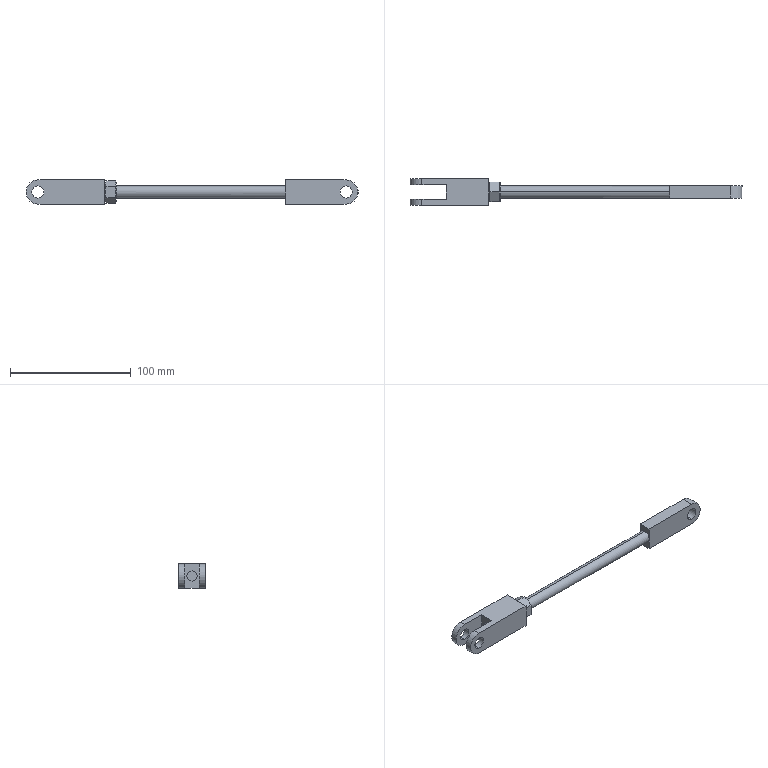Part | SolidWorks | features MirrorStock 1 | 3 solids | 42 faces | box 275 x 22 x 20 mm | volume 44683 mm3 | plane 23 | cylinder 15 | cone 4 | commonest cylinder face diameters 10 x8 20 x3 8.376 x2 8.5 x2
STEP:
#1=CARTESIAN_POINT('',(20.,0.,4.25));
#2=VERTEX_POINT('',#1);
#3=CARTESIAN_POINT('',(20.,0.,-4.25));
#4=VERTEX_POINT('',#3);
#5=CARTESIAN_POINT('',(20.,0.,0.));
#6=DIRECTION('',(-1.,0.,0.));
#7=DIRECTION('',(0.,0.,1.));
#8=AXIS2_PLACEMENT_3D('',#5,#6,#7);
#9=CIRCLE('',#8,4.25);
#10=EDGE_CURVE('',#2,#4,#9,.T.);
#11=ORIENTED_EDGE('',*,*,#10,.T.);
#12=CARTESIAN_POINT('',(55.,0.,-4.25));
#13=VERTEX_POINT('',#12);
#14=CARTESIAN_POINT('',(55.,0.,-4.25));
#15=DIRECTION('',(1.,0.,0.));
#16=VECTOR('',#15,1000.);
#17=LINE('',#14,#16);
#18=EDGE_CURVE('',#4,#13,#17,.T.);
#19=ORIENTED_EDGE('',*,*,#18,.T.);
#20=CARTESIAN_POINT('',(55.,0.,4.25));
#21=VERTEX_POINT('',#20);
#22=CARTESIAN_POINT('',(55.,0.,0.));
#23=DIRECTION('',(-1.,0.,0.));
#24=DIRECTION('',(0.,0.,1.));
#25=AXIS2_PLACEMENT_3D('',#22,#23,#24);
#26=CIRCLE('',#25,4.25);
#27=EDGE_CURVE('',#21,#13,#26,.T.);
#28=ORIENTED_EDGE('',*,*,#27,.F.);
#29=CARTESIAN_POINT('',(55.,0.,4.25));
#30=DIRECTION('',(1.,0.,0.));
#31=VECTOR('',#30,1000.);
#32=LINE('',#29,#31);
#33=EDGE_CURVE('',#2,#21,#32,.T.);
#34=ORIENTED_EDGE('',*,*,#33,.F.);
#35=EDGE_LOOP('',(#11,#19,#28,#34));
#36=FACE_OUTER_BOUND('',#35,.T.);
#37=CARTESIAN_POINT('',(55.,0.,0.));
#38=DIRECTION('',(1.,0.,0.));
#39=DIRECTION('',(0.,0.,1.));
#40=AXIS2_PLACEMENT_3D('',#37,#38,#39);
#41=CYLINDRICAL_SURFACE('',#40,4.25);
#42=ADVANCED_FACE('',(#36),#41,.F.);
#43=CARTESIAN_POINT('',(0.,11.,-5.));
#44=VERTEX_POINT('',#43);
#45=CARTESIAN_POINT('',(0.,11.,5.));
#46=VERTEX_POINT('',#45);
#47=CARTESIAN_POINT('',(0.,11.,0.));
#48=DIRECTION('',(0.,-1.,0.));
#49=DIRECTION('',(0.,0.,-1.));
#50=AXIS2_PLACEMENT_3D('',#47,#48,#49);
#51=CIRCLE('',#50,5.);
#52=EDGE_CURVE('',#44,#46,#51,.T.);
#53=ORIENTED_EDGE('',*,*,#52,.F.);
#54=CARTESIAN_POINT('',(0.,6.,-5.));
#55=VERTEX_POINT('',#54);
#56=CARTESIAN_POINT('',(0.,11.,-5.));
#57=DIRECTION('',(0.,-1.,0.));
#58=VECTOR('',#57,1000.);
#59=LINE('',#56,#58);
#60=EDGE_CURVE('',#44,#55,#59,.T.);
#61=ORIENTED_EDGE('',*,*,#60,.T.);
#62=CARTESIAN_POINT('',(0.,6.,5.));
#63=VERTEX_POINT('',#62);
#64=CARTESIAN_POINT('',(0.,6.,0.));
#65=DIRECTION('',(0.,-1.,0.));
#66=DIRECTION('',(0.,0.,-1.));
#67=AXIS2_PLACEMENT_3D('',#64,#65,#66);
#68=CIRCLE('',#67,5.);
#69=EDGE_CURVE('',#55,#63,#68,.T.);
#70=ORIENTED_EDGE('',*,*,#69,.T.);
#71=CARTESIAN_POINT('',(0.,11.,5.));
#72=DIRECTION('',(0.,-1.,0.));
#73=VECTOR('',#72,1000.);
#74=LINE('',#71,#73);
#75=EDGE_CURVE('',#46,#63,#74,.T.);
#76=ORIENTED_EDGE('',*,*,#75,.F.);
#77=EDGE_LOOP('',(#53,#61,#70,#76));
#78=FACE_OUTER_BOUND('',#77,.T.);
#79=CARTESIAN_POINT('',(0.,11.,0.));
#80=DIRECTION('',(0.,-1.,0.));
#81=DIRECTION('',(0.,0.,1.));
#82=AXIS2_PLACEMENT_3D('',#79,#80,#81);
#83=CYLINDRICAL_SURFACE('',#82,5.);
#84=ADVANCED_FACE('',(#78),#83,.F.);
#85=CARTESIAN_POINT('',(0.,-6.,5.));
#86=VERTEX_POINT('',#85);
#87=CARTESIAN_POINT('',(0.,-6.,-5.));
#88=VERTEX_POINT('',#87);
#89=CARTESIAN_POINT('',(0.,-6.,0.));
#90=DIRECTION('',(0.,1.,0.));
#91=DIRECTION('',(0.,0.,1.));
#92=AXIS2_PLACEMENT_3D('',#89,#90,#91);
#93=CIRCLE('',#92,5.);
#94=EDGE_CURVE('',#86,#88,#93,.T.);
#95=ORIENTED_EDGE('',*,*,#94,.T.);
#96=CARTESIAN_POINT('',(0.,-11.,-5.));
#97=VERTEX_POINT('',#96);
#98=CARTESIAN_POINT('',(0.,11.,-5.));
#99=DIRECTION('',(0.,-1.,0.));
#100=VECTOR('',#99,1000.);
#101=LINE('',#98,#100);
#102=EDGE_CURVE('',#88,#97,#101,.T.);
#103=ORIENTED_EDGE('',*,*,#102,.T.);
#104=CARTESIAN_POINT('',(0.,-11.,5.));
#105=VERTEX_POINT('',#104);
#106=CARTESIAN_POINT('',(0.,-11.,0.));
#107=DIRECTION('',(0.,-1.,0.));
#108=DIRECTION('',(0.,0.,-1.));
#109=AXIS2_PLACEMENT_3D('',#106,#107,#108);
#110=CIRCLE('',#109,5.);
#111=EDGE_CURVE('',#97,#105,#110,.T.);
#112=ORIENTED_EDGE('',*,*,#111,.T.);
#113=CARTESIAN_POINT('',(0.,11.,5.));
#114=DIRECTION('',(0.,-1.,0.));
#115=VECTOR('',#114,1000.);
#116=LINE('',#113,#115);
#117=EDGE_CURVE('',#86,#105,#116,.T.);
#118=ORIENTED_EDGE('',*,*,#117,.F.);
#119=EDGE_LOOP('',(#95,#103,#112,#118));
#120=FACE_OUTER_BOUND('',#119,.T.);
#121=CARTESIAN_POINT('',(0.,11.,0.));
#122=DIRECTION('',(0.,-1.,0.));
#123=DIRECTION('',(0.,0.,1.));
#124=AXIS2_PLACEMENT_3D('',#121,#122,#123);
#125=CYLINDRICAL_SURFACE('',#124,5.);
#126=ADVANCED_FACE('',(#120),#125,.F.);
#127=CARTESIAN_POINT('',(0.,-6.,-10.));
#128=VERTEX_POINT('',#127);
#129=CARTESIAN_POINT('',(0.,-11.,-10.));
#130=VERTEX_POINT('',#129);
#131=CARTESIAN_POINT('',(0.,11.,-10.));
#132=DIRECTION('',(0.,-1.,0.));
#133=VECTOR('',#132,1000.);
#134=LINE('',#131,#133);
#135=EDGE_CURVE('',#128,#130,#134,.T.);
#136=ORIENTED_EDGE('',*,*,#135,.T.);
#137=CARTESIAN_POINT('',(0.,-11.,10.));
#138=VERTEX_POINT('',#137);
#139=CARTESIAN_POINT('',(0.,-11.,0.));
#140=DIRECTION('',(0.,-1.,0.));
#141=DIRECTION('',(0.,0.,-1.));
#142=AXIS2_PLACEMENT_3D('',#139,#140,#141);
#143=CIRCLE('',#142,10.);
#144=EDGE_CURVE('',#138,#130,#143,.T.);
#145=ORIENTED_EDGE('',*,*,#144,.F.);
#146=CARTESIAN_POINT('',(0.,-6.,10.));
#147=VERTEX_POINT('',#146);
#148=CARTESIAN_POINT('',(0.,11.,10.));
#149=DIRECTION('',(0.,-1.,0.));
#150=VECTOR('',#149,1000.);
#151=LINE('',#148,#150);
#152=EDGE_CURVE('',#147,#138,#151,.T.);
#153=ORIENTED_EDGE('',*,*,#152,.F.);
#154=CARTESIAN_POINT('',(0.,-6.,0.));
#155=DIRECTION('',(0.,1.,0.));
#156=DIRECTION('',(0.,0.,1.));
#157=AXIS2_PLACEMENT_3D('',#154,#155,#156);
#158=CIRCLE('',#157,10.);
#159=EDGE_CURVE('',#128,#147,#158,.T.);
#160=ORIENTED_EDGE('',*,*,#159,.F.);
#161=EDGE_LOOP('',(#136,#145,#153,#160));
#162=FACE_OUTER_BOUND('',#161,.T.);
#163=CARTESIAN_POINT('',(0.,11.,0.));
#164=DIRECTION('',(0.,-1.,0.));
#165=DIRECTION('',(0.,0.,1.));
#166=AXIS2_PLACEMENT_3D('',#163,#164,#165);
#167=CYLINDRICAL_SURFACE('',#166,10.);
#168=ADVANCED_FACE('',(#162),#167,.T.);
#169=ORIENTED_EDGE('',*,*,#102,.F.);
#170=CARTESIAN_POINT('',(0.,-6.,0.));
#171=DIRECTION('',(0.,1.,0.));
#172=DIRECTION('',(0.,0.,1.));
#173=AXIS2_PLACEMENT_3D('',#170,#171,#172);
#174=CIRCLE('',#173,5.);
#175=EDGE_CURVE('',#88,#86,#174,.T.);
#176=ORIENTED_EDGE('',*,*,#175,.T.);
#177=ORIENTED_EDGE('',*,*,#117,.T.);
#178=CARTESIAN_POINT('',(0.,-11.,0.));
#179=DIRECTION('',(0.,-1.,0.));
#180=DIRECTION('',(0.,0.,-1.));
#181=AXIS2_PLACEMENT_3D('',#178,#179,#180);
#182=CIRCLE('',#181,5.);
#183=EDGE_CURVE('',#105,#97,#182,.T.);
#184=ORIENTED_EDGE('',*,*,#183,.T.);
#185=EDGE_LOOP('',(#169,#176,#177,#184));
#186=FACE_OUTER_BOUND('',#185,.T.);
#187=CARTESIAN_POINT('',(0.,11.,0.));
#188=DIRECTION('',(0.,-1.,0.));
#189=DIRECTION('',(0.,0.,1.));
#190=AXIS2_PLACEMENT_3D('',#187,#188,#189);
#191=CYLINDRICAL_SURFACE('',#190,5.);
#192=ADVANCED_FACE('',(#186),#191,.F.);
#193=CARTESIAN_POINT('',(0.,11.,10.));
#194=VERTEX_POINT('',#193);
#195=CARTESIAN_POINT('',(0.,11.,-10.));
#196=VERTEX_POINT('',#195);
#197=CARTESIAN_POINT('',(0.,11.,0.));
#198=DIRECTION('',(0.,-1.,0.));
#199=DIRECTION('',(0.,0.,-1.));
#200=AXIS2_PLACEMENT_3D('',#197,#198,#199);
#201=CIRCLE('',#200,10.);
#202=EDGE_CURVE('',#194,#196,#201,.T.);
#203=ORIENTED_EDGE('',*,*,#202,.F.);
#204=CARTESIAN_POINT('',(55.,11.,10.));
#205=VERTEX_POINT('',#204);
#206=CARTESIAN_POINT('',(0.,11.,10.));
#207=DIRECTION('',(-1.,0.,0.));
#208=VECTOR('',#207,1000.);
#209=LINE('',#206,#208);
#210=EDGE_CURVE('',#205,#194,#209,.T.);
#211=ORIENTED_EDGE('',*,*,#210,.F.);
#212=CARTESIAN_POINT('',(55.,11.,-10.));
#213=VERTEX_POINT('',#212);
#214=CARTESIAN_POINT('',(55.,11.,10.));
#215=DIRECTION('',(0.,0.,1.));
#216=VECTOR('',#215,1000.);
#217=LINE('',#214,#216);
#218=EDGE_CURVE('',#213,#205,#217,.T.);
#219=ORIENTED_EDGE('',*,*,#218,.F.);
#220=CARTESIAN_POINT('',(0.,11.,-10.));
#221=DIRECTION('',(1.,0.,0.));
#222=VECTOR('',#221,1000.);
#223=LINE('',#220,#222);
#224=EDGE_CURVE('',#196,#213,#223,.T.);
#225=ORIENTED_EDGE('',*,*,#224,.F.);
#226=EDGE_LOOP('',(#203,#211,#219,#225));
#227=FACE_OUTER_BOUND('',#226,.T.);
#228=CARTESIAN_POINT('',(0.,11.,0.));
#229=DIRECTION('',(0.,-1.,0.));
#230=DIRECTION('',(0.,0.,-1.));
#231=AXIS2_PLACEMENT_3D('',#228,#229,#230);
#232=CIRCLE('',#231,5.);
#233=EDGE_CURVE('',#46,#44,#232,.T.);
#234=ORIENTED_EDGE('',*,*,#233,.T.);
#235=ORIENTED_EDGE('',*,*,#52,.T.);
#236=EDGE_LOOP('',(#234,#235));
#237=FACE_BOUND('',#236,.T.);
#238=CARTESIAN_POINT('',(0.,11.,0.));
#239=DIRECTION('',(0.,1.,0.));
#240=DIRECTION('',(0.,0.,-1.));
#241=AXIS2_PLACEMENT_3D('',#238,#239,#240);
#242=PLANE('',#241);
#243=ADVANCED_FACE('',(#227,#237),#242,.T.);
#244=ORIENTED_EDGE('',*,*,#144,.T.);
#245=CARTESIAN_POINT('',(55.,-11.,-10.));
#246=VERTEX_POINT('',#245);
#247=CARTESIAN_POINT('',(0.,-11.,-10.));
#248=DIRECTION('',(1.,0.,0.));
#249=VECTOR('',#248,1000.);
#250=LINE('',#247,#249);
#251=EDGE_CURVE('',#130,#246,#250,.T.);
#252=ORIENTED_EDGE('',*,*,#251,.T.);
#253=CARTESIAN_POINT('',(55.,-11.,10.));
#254=VERTEX_POINT('',#253);
#255=CARTESIAN_POINT('',(55.,-11.,10.));
#256=DIRECTION('',(0.,0.,1.));
#257=VECTOR('',#256,1000.);
#258=LINE('',#255,#257);
#259=EDGE_CURVE('',#246,#254,#258,.T.);
#260=ORIENTED_EDGE('',*,*,#259,.T.);
#261=CARTESIAN_POINT('',(0.,-11.,10.));
#262=DIRECTION('',(-1.,0.,0.));
#263=VECTOR('',#262,1000.);
#264=LINE('',#261,#263);
#265=EDGE_CURVE('',#254,#138,#264,.T.);
#266=ORIENTED_EDGE('',*,*,#265,.T.);
#267=EDGE_LOOP('',(#244,#252,#260,#266));
#268=FACE_OUTER_BOUND('',#267,.T.);
#269=ORIENTED_EDGE('',*,*,#183,.F.);
#270=ORIENTED_EDGE('',*,*,#111,.F.);
#271=EDGE_LOOP('',(#269,#270));
#272=FACE_BOUND('',#271,.T.);
#273=CARTESIAN_POINT('',(0.,-11.,0.));
#274=DIRECTION('',(0.,1.,0.));
#275=DIRECTION('',(0.,0.,-1.));
#276=AXIS2_PLACEMENT_3D('',#273,#274,#275);
#277=PLANE('',#276);
#278=ADVANCED_FACE('',(#268,#272),#277,.F.);
#279=CARTESIAN_POINT('',(0.,6.,10.));
#280=VERTEX_POINT('',#279);
#281=CARTESIAN_POINT('',(0.,11.,10.));
#282=DIRECTION('',(0.,-1.,0.));
#283=VECTOR('',#282,1000.);
#284=LINE('',#281,#283);
#285=EDGE_CURVE('',#194,#280,#284,.T.);
#286=ORIENTED_EDGE('',*,*,#285,.F.);
#287=ORIENTED_EDGE('',*,*,#202,.T.);
#288=CARTESIAN_POINT('',(0.,6.,-10.));
#289=VERTEX_POINT('',#288);
#290=CARTESIAN_POINT('',(0.,11.,-10.));
#291=DIRECTION('',(0.,-1.,0.));
#292=VECTOR('',#291,1000.);
#293=LINE('',#290,#292);
#294=EDGE_CURVE('',#196,#289,#293,.T.);
#295=ORIENTED_EDGE('',*,*,#294,.T.);
#296=CARTESIAN_POINT('',(0.,6.,0.));
#297=DIRECTION('',(0.,-1.,0.));
#298=DIRECTION('',(0.,0.,-1.));
#299=AXIS2_PLACEMENT_3D('',#296,#297,#298);
#300=CIRCLE('',#299,10.);
#301=EDGE_CURVE('',#280,#289,#300,.T.);
#302=ORIENTED_EDGE('',*,*,#301,.F.);
#303=EDGE_LOOP('',(#286,#287,#295,#302));
#304=FACE_OUTER_BOUND('',#303,.T.);
#305=CARTESIAN_POINT('',(0.,11.,0.));
#306=DIRECTION('',(0.,-1.,0.));
#307=DIRECTION('',(0.,0.,1.));
#308=AXIS2_PLACEMENT_3D('',#305,#306,#307);
#309=CYLINDRICAL_SURFACE('',#308,10.);
#310=ADVANCED_FACE('',(#304),#309,.T.);
#311=CARTESIAN_POINT('',(20.,-6.,-10.));
#312=VERTEX_POINT('',#311);
#313=CARTESIAN_POINT('',(20.,6.,-10.));
#314=VERTEX_POINT('',#313);
#315=CARTESIAN_POINT('',(20.,-6.,-10.));
#316=DIRECTION('',(0.,1.,0.));
#317=VECTOR('',#316,1000.);
#318=LINE('',#315,#317);
#319=EDGE_CURVE('',#312,#314,#318,.T.);
#320=ORIENTED_EDGE('',*,*,#319,.T.);
#321=CARTESIAN_POINT('',(-20.,6.,-10.));
#322=DIRECTION('',(-1.,0.,0.));
#323=VECTOR('',#322,1000.);
#324=LINE('',#321,#323);
#325=EDGE_CURVE('',#314,#289,#324,.T.);
#326=ORIENTED_EDGE('',*,*,#325,.T.);
#327=ORIENTED_EDGE('',*,*,#294,.F.);
#328=ORIENTED_EDGE('',*,*,#224,.T.);
#329=CARTESIAN_POINT('',(55.,11.,-10.));
#330=DIRECTION('',(0.,-1.,0.));
#331=VECTOR('',#330,1000.);
#332=LINE('',#329,#331);
#333=EDGE_CURVE('',#213,#246,#332,.T.);
#334=ORIENTED_EDGE('',*,*,#333,.T.);
#335=ORIENTED_EDGE('',*,*,#251,.F.);
#336=ORIENTED_EDGE('',*,*,#135,.F.);
#337=CARTESIAN_POINT('',(-20.,-6.,-10.));
#338=DIRECTION('',(1.,0.,0.));
#339=VECTOR('',#338,1000.);
#340=LINE('',#337,#339);
#341=EDGE_CURVE('',#128,#312,#340,.T.);
#342=ORIENTED_EDGE('',*,*,#341,.T.);
#343=EDGE_LOOP('',(#320,#326,#327,#328,#334,#335,#336,#342));
#344=FACE_OUTER_BOUND('',#343,.T.);
#345=CARTESIAN_POINT('',(0.,11.,-10.));
#346=DIRECTION('',(0.,0.,1.));
#347=DIRECTION('',(-1.,0.,0.));
#348=AXIS2_PLACEMENT_3D('',#345,#346,#347);
#349=PLANE('',#348);
#350=ADVANCED_FACE('',(#344),#349,.F.);
#351=ORIENTED_EDGE('',*,*,#27,.T.);
#352=CARTESIAN_POINT('',(55.,0.,0.));
#353=DIRECTION('',(-1.,0.,0.));
#354=DIRECTION('',(0.,0.,1.));
#355=AXIS2_PLACEMENT_3D('',#352,#353,#354);
#356=CIRCLE('',#355,4.25);
#357=EDGE_CURVE('',#13,#21,#356,.T.);
#358=ORIENTED_EDGE('',*,*,#357,.T.);
#359=EDGE_LOOP('',(#351,#358));
#360=FACE_BOUND('',#359,.T.);
#361=ORIENTED_EDGE('',*,*,#259,.F.);
#362=ORIENTED_EDGE('',*,*,#333,.F.);
#363=ORIENTED_EDGE('',*,*,#218,.T.);
#364=CARTESIAN_POINT('',(55.,11.,10.));
#365=DIRECTION('',(0.,-1.,0.));
#366=VECTOR('',#365,1000.);
#367=LINE('',#364,#366);
#368=EDGE_CURVE('',#205,#254,#367,.T.);
#369=ORIENTED_EDGE('',*,*,#368,.T.);
#370=EDGE_LOOP('',(#361,#362,#363,#369));
#371=FACE_OUTER_BOUND('',#370,.T.);
#372=CARTESIAN_POINT('',(55.,11.,10.));
#373=DIRECTION('',(-1.,0.,0.));
#374=DIRECTION('',(0.,0.,-1.));
#375=AXIS2_PLACEMENT_3D('',#372,#373,#374);
#376=PLANE('',#375);
#377=ADVANCED_FACE('',(#360,#371),#376,.F.);
#378=ORIENTED_EDGE('',*,*,#152,.T.);
#379=ORIENTED_EDGE('',*,*,#265,.F.);
#380=ORIENTED_EDGE('',*,*,#368,.F.);
#381=ORIENTED_EDGE('',*,*,#210,.T.);
#382=ORIENTED_EDGE('',*,*,#285,.T.);
#383=CARTESIAN_POINT('',(20.,6.,10.));
#384=VERTEX_POINT('',#383);
#385=CARTESIAN_POINT('',(-20.,6.,10.));
#386=DIRECTION('',(-1.,0.,0.));
#387=VECTOR('',#386,1000.);
#388=LINE('',#385,#387);
#389=EDGE_CURVE('',#384,#280,#388,.T.);
#390=ORIENTED_EDGE('',*,*,#389,.F.);
#391=CARTESIAN_POINT('',(20.,-6.,10.));
#392=VERTEX_POINT('',#391);
#393=CARTESIAN_POINT('',(20.,-6.,10.));
#394=DIRECTION('',(0.,1.,0.));
#395=VECTOR('',#394,1000.);
#396=LINE('',#393,#395);
#397=EDGE_CURVE('',#392,#384,#396,.T.);
#398=ORIENTED_EDGE('',*,*,#397,.F.);
#399=CARTESIAN_POINT('',(-20.,-6.,10.));
#400=DIRECTION('',(1.,0.,0.));
#401=VECTOR('',#400,1000.);
#402=LINE('',#399,#401);
#403=EDGE_CURVE('',#147,#392,#402,.T.);
#404=ORIENTED_EDGE('',*,*,#403,.F.);
#405=EDGE_LOOP('',(#378,#379,#380,#381,#382,#390,#398,#404));
#406=FACE_OUTER_BOUND('',#405,.T.);
#407=CARTESIAN_POINT('',(0.,11.,10.));
#408=DIRECTION('',(0.,0.,-1.));
#409=DIRECTION('',(1.,0.,0.));
#410=AXIS2_PLACEMENT_3D('',#407,#408,#409);
#411=PLANE('',#410);
#412=ADVANCED_FACE('',(#406),#411,.F.);
#413=ORIENTED_EDGE('',*,*,#60,.F.);
#414=ORIENTED_EDGE('',*,*,#233,.F.);
#415=ORIENTED_EDGE('',*,*,#75,.T.);
#416=CARTESIAN_POINT('',(0.,6.,0.));
#417=DIRECTION('',(0.,-1.,0.));
#418=DIRECTION('',(0.,0.,-1.));
#419=AXIS2_PLACEMENT_3D('',#416,#417,#418);
#420=CIRCLE('',#419,5.);
#421=EDGE_CURVE('',#63,#55,#420,.T.);
#422=ORIENTED_EDGE('',*,*,#421,.T.);
#423=EDGE_LOOP('',(#413,#414,#415,#422));
#424=FACE_OUTER_BOUND('',#423,.T.);
#425=CARTESIAN_POINT('',(0.,11.,0.));
#426=DIRECTION('',(0.,-1.,0.));
#427=DIRECTION('',(0.,0.,1.));
#428=AXIS2_PLACEMENT_3D('',#425,#426,#427);
#429=CYLINDRICAL_SURFACE('',#428,5.);
#430=ADVANCED_FACE('',(#424),#429,.F.);
#431=ORIENTED_EDGE('',*,*,#94,.F.);
#432=ORIENTED_EDGE('',*,*,#175,.F.);
#433=EDGE_LOOP('',(#431,#432));
#434=FACE_BOUND('',#433,.T.);
#435=ORIENTED_EDGE('',*,*,#341,.F.);
#436=ORIENTED_EDGE('',*,*,#159,.T.);
#437=ORIENTED_EDGE('',*,*,#403,.T.);
#438=CARTESIAN_POINT('',(20.,-6.,10.));
#439=DIRECTION('',(0.,0.,-1.));
#440=VECTOR('',#439,1000.);
#441=LINE('',#438,#440);
#442=EDGE_CURVE('',#392,#312,#441,.T.);
#443=ORIENTED_EDGE('',*,*,#442,.T.);
#444=EDGE_LOOP('',(#435,#436,#437,#443));
#445=FACE_OUTER_BOUND('',#444,.T.);
#446=CARTESIAN_POINT('',(-20.,-6.,10.));
#447=DIRECTION('',(0.,-1.,0.));
#448=DIRECTION('',(0.,0.,1.));
#449=AXIS2_PLACEMENT_3D('',#446,#447,#448);
#450=PLANE('',#449);
#451=ADVANCED_FACE('',(#434,#445),#450,.F.);
#452=ORIENTED_EDGE('',*,*,#421,.F.);
#453=ORIENTED_EDGE('',*,*,#69,.F.);
#454=EDGE_LOOP('',(#452,#453));
#455=FACE_BOUND('',#454,.T.);
#456=ORIENTED_EDGE('',*,*,#389,.T.);
#457=ORIENTED_EDGE('',*,*,#301,.T.);
#458=ORIENTED_EDGE('',*,*,#325,.F.);
#459=CARTESIAN_POINT('',(20.,6.,10.));
#460=DIRECTION('',(0.,0.,-1.));
#461=VECTOR('',#460,1000.);
#462=LINE('',#459,#461);
#463=EDGE_CURVE('',#384,#314,#462,.T.);
#464=ORIENTED_EDGE('',*,*,#463,.F.);
#465=EDGE_LOOP('',(#456,#457,#458,#464));
#466=FACE_OUTER_BOUND('',#465,.T.);
#467=CARTESIAN_POINT('',(-20.,6.,10.));
#468=DIRECTION('',(0.,1.,0.));
#469=DIRECTION('',(0.,0.,-1.));
#470=AXIS2_PLACEMENT_3D('',#467,#468,#469);
#471=PLANE('',#470);
#472=ADVANCED_FACE('',(#455,#466),#471,.F.);
#473=ORIENTED_EDGE('',*,*,#10,.F.);
#474=CARTESIAN_POINT('',(20.,0.,0.));
#475=DIRECTION('',(-1.,0.,0.));
#476=DIRECTION('',(0.,0.,1.));
#477=AXIS2_PLACEMENT_3D('',#474,#475,#476);
#478=CIRCLE('',#477,4.25);
#479=EDGE_CURVE('',#4,#2,#478,.T.);
#480=ORIENTED_EDGE('',*,*,#479,.F.);
#481=EDGE_LOOP('',(#473,#480));
#482=FACE_BOUND('',#481,.T.);
#483=ORIENTED_EDGE('',*,*,#463,.T.);
#484=ORIENTED_EDGE('',*,*,#319,.F.);
#485=ORIENTED_EDGE('',*,*,#442,.F.);
#486=ORIENTED_EDGE('',*,*,#397,.T.);
#487=EDGE_LOOP('',(#483,#484,#485,#486));
#488=FACE_OUTER_BOUND('',#487,.T.);
#489=CARTESIAN_POINT('',(20.,-6.,10.));
#490=DIRECTION('',(1.,0.,0.));
#491=DIRECTION('',(0.,0.,1.));
#492=AXIS2_PLACEMENT_3D('',#489,#490,#491);
#493=PLANE('',#492);
#494=ADVANCED_FACE('',(#482,#488),#493,.F.);
#495=ORIENTED_EDGE('',*,*,#18,.F.);
#496=ORIENTED_EDGE('',*,*,#479,.T.);
#497=ORIENTED_EDGE('',*,*,#33,.T.);
#498=ORIENTED_EDGE('',*,*,#357,.F.);
#499=EDGE_LOOP('',(#495,#496,#497,#498));
#500=FACE_OUTER_BOUND('',#499,.T.);
#501=CARTESIAN_POINT('',(55.,0.,0.));
#502=DIRECTION('',(1.,0.,0.));
#503=DIRECTION('',(0.,0.,1.));
#504=AXIS2_PLACEMENT_3D('',#501,#502,#503);
#505=CYLINDRICAL_SURFACE('',#504,4.25);
#506=ADVANCED_FACE('',(#500),#505,.F.);
#507=CLOSED_SHELL('',(#42,#84,#126,#168,#192,#243,#278,#310,#350,#377,#412,#430,#451,#472,#494,#506));
#508=MANIFOLD_SOLID_BREP('',#507);
#509=CARTESIAN_POINT('',(255.,5.,-5.));
#510=VERTEX_POINT('',#509);
#511=CARTESIAN_POINT('',(255.,5.,5.));
#512=VERTEX_POINT('',#511);
#513=CARTESIAN_POINT('',(255.,5.,0.));
#514=DIRECTION('',(0.,-1.,0.));
#515=DIRECTION('',(0.,0.,-1.));
#516=AXIS2_PLACEMENT_3D('',#513,#514,#515);
#517=CIRCLE('',#516,5.);
#518=EDGE_CURVE('',#510,#512,#517,.T.);
#519=ORIENTED_EDGE('',*,*,#518,.F.);
#520=CARTESIAN_POINT('',(255.,-5.,-5.));
#521=VERTEX_POINT('',#520);
#522=CARTESIAN_POINT('',(255.,5.,-5.));
#523=DIRECTION('',(0.,-1.,0.));
#524=VECTOR('',#523,1000.);
#525=LINE('',#522,#524);
#526=EDGE_CURVE('',#510,#521,#525,.T.);
#527=ORIENTED_EDGE('',*,*,#526,.T.);
#528=CARTESIAN_POINT('',(255.,-5.,5.));
#529=VERTEX_POINT('',#528);
#530=CARTESIAN_POINT('',(255.,-5.,0.));
#531=DIRECTION('',(0.,-1.,0.));
#532=DIRECTION('',(0.,0.,-1.));
#533=AXIS2_PLACEMENT_3D('',#530,#531,#532);
#534=CIRCLE('',#533,5.);
#535=EDGE_CURVE('',#521,#529,#534,.T.);
#536=ORIENTED_EDGE('',*,*,#535,.T.);
#537=CARTESIAN_POINT('',(255.,5.,5.));
#538=DIRECTION('',(0.,-1.,0.));
#539=VECTOR('',#538,1000.);
#540=LINE('',#537,#539);
#541=EDGE_CURVE('',#512,#529,#540,.T.);
#542=ORIENTED_EDGE('',*,*,#541,.F.);
#543=EDGE_LOOP('',(#519,#527,#536,#542));
#544=FACE_OUTER_BOUND('',#543,.T.);
#545=CARTESIAN_POINT('',(255.,5.,0.));
#546=DIRECTION('',(0.,-1.,0.));
#547=DIRECTION('',(0.,0.,1.));
#548=AXIS2_PLACEMENT_3D('',#545,#546,#547);
#549=CYLINDRICAL_SURFACE('',#548,5.);
#550=ADVANCED_FACE('',(#544),#549,.F.);
#551=CARTESIAN_POINT('',(205.,-5.,0.));
#552=VERTEX_POINT('',#551);
#553=CARTESIAN_POINT('',(205.,0.,5.));
#554=VERTEX_POINT('',#553);
#555=CARTESIAN_POINT('',(205.,0.,0.));
#556=DIRECTION('',(-1.,0.,0.));
#557=DIRECTION('',(0.,0.,1.));
#558=AXIS2_PLACEMENT_3D('',#555,#556,#557);
#559=CIRCLE('',#558,5.);
#560=EDGE_CURVE('',#552,#554,#559,.T.);
#561=ORIENTED_EDGE('',*,*,#560,.T.);
#562=CARTESIAN_POINT('',(25.,0.,5.));
#563=VERTEX_POINT('',#562);
#564=CARTESIAN_POINT('',(205.,0.,5.));
#565=DIRECTION('',(-1.,0.,0.));
#566=VECTOR('',#565,1000.);
#567=LINE('',#564,#566);
#568=EDGE_CURVE('',#554,#563,#567,.T.);
#569=ORIENTED_EDGE('',*,*,#568,.T.);
#570=CARTESIAN_POINT('',(25.,0.,-5.));
#571=VERTEX_POINT('',#570);
#572=CARTESIAN_POINT('',(25.,0.,0.));
#573=DIRECTION('',(-1.,0.,0.));
#574=DIRECTION('',(0.,0.,1.));
#575=AXIS2_PLACEMENT_3D('',#572,#573,#574);
#576=CIRCLE('',#575,5.);
#577=EDGE_CURVE('',#571,#563,#576,.T.);
#578=ORIENTED_EDGE('',*,*,#577,.F.);
#579=CARTESIAN_POINT('',(205.,0.,-5.));
#580=VERTEX_POINT('',#579);
#581=CARTESIAN_POINT('',(205.,0.,-5.));
#582=DIRECTION('',(-1.,0.,0.));
#583=VECTOR('',#582,1000.);
#584=LINE('',#581,#583);
#585=EDGE_CURVE('',#580,#571,#584,.T.);
#586=ORIENTED_EDGE('',*,*,#585,.F.);
#587=CARTESIAN_POINT('',(205.,0.,0.));
#588=DIRECTION('',(-1.,0.,0.));
#589=DIRECTION('',(0.,0.,1.));
#590=AXIS2_PLACEMENT_3D('',#587,#588,#589);
#591=CIRCLE('',#590,5.);
#592=EDGE_CURVE('',#580,#552,#591,.T.);
#593=ORIENTED_EDGE('',*,*,#592,.T.);
#594=EDGE_LOOP('',(#561,#569,#578,#586,#593));
#595=FACE_OUTER_BOUND('',#594,.T.);
#596=CARTESIAN_POINT('',(205.,0.,0.));
#597=DIRECTION('',(-1.,0.,0.));
#598=DIRECTION('',(0.,0.,-1.));
#599=AXIS2_PLACEMENT_3D('',#596,#597,#598);
#600=CYLINDRICAL_SURFACE('',#599,5.);
#601=ADVANCED_FACE('',(#595),#600,.T.);
#602=ORIENTED_EDGE('',*,*,#568,.F.);
#603=CARTESIAN_POINT('',(205.,5.,0.));
#604=VERTEX_POINT('',#603);
#605=CARTESIAN_POINT('',(205.,0.,0.));
#606=DIRECTION('',(-1.,0.,0.));
#607=DIRECTION('',(0.,0.,1.));
#608=AXIS2_PLACEMENT_3D('',#605,#606,#607);
#609=CIRCLE('',#608,5.);
#610=EDGE_CURVE('',#554,#604,#609,.T.);
#611=ORIENTED_EDGE('',*,*,#610,.T.);
#612=CARTESIAN_POINT('',(205.,0.,0.));
#613=DIRECTION('',(-1.,0.,0.));
#614=DIRECTION('',(0.,0.,1.));
#615=AXIS2_PLACEMENT_3D('',#612,#613,#614);
#616=CIRCLE('',#615,5.);
#617=EDGE_CURVE('',#604,#580,#616,.T.);
#618=ORIENTED_EDGE('',*,*,#617,.T.);
#619=ORIENTED_EDGE('',*,*,#585,.T.);
#620=CARTESIAN_POINT('',(25.,0.,0.));
#621=DIRECTION('',(-1.,0.,0.));
#622=DIRECTION('',(0.,0.,1.));
#623=AXIS2_PLACEMENT_3D('',#620,#621,#622);
#624=CIRCLE('',#623,5.);
#625=EDGE_CURVE('',#563,#571,#624,.T.);
#626=ORIENTED_EDGE('',*,*,#625,.F.);
#627=EDGE_LOOP('',(#602,#611,#618,#619,#626));
#628=FACE_OUTER_BOUND('',#627,.T.);
#629=CARTESIAN_POINT('',(205.,0.,0.));
#630=DIRECTION('',(-1.,0.,0.));
#631=DIRECTION('',(0.,0.,-1.));
#632=AXIS2_PLACEMENT_3D('',#629,#630,#631);
#633=CYLINDRICAL_SURFACE('',#632,5.);
#634=ADVANCED_FACE('',(#628),#633,.T.);
#635=ORIENTED_EDGE('',*,*,#577,.T.);
#636=ORIENTED_EDGE('',*,*,#625,.T.);
#637=EDGE_LOOP('',(#635,#636));
#638=FACE_OUTER_BOUND('',#637,.T.);
#639=CARTESIAN_POINT('',(25.,0.,0.));
#640=DIRECTION('',(1.,0.,0.));
#641=DIRECTION('',(0.,0.,1.));
#642=AXIS2_PLACEMENT_3D('',#639,#640,#641);
#643=PLANE('',#642);
#644=ADVANCED_FACE('',(#638),#643,.F.);
#645=CARTESIAN_POINT('',(205.,5.,-10.));
#646=VERTEX_POINT('',#645);
#647=CARTESIAN_POINT('',(205.,5.,-10.));
#648=DIRECTION('',(0.,0.,-1.));
#649=VECTOR('',#648,1000.);
#650=LINE('',#647,#649);
#651=EDGE_CURVE('',#604,#646,#650,.T.);
#652=ORIENTED_EDGE('',*,*,#651,.T.);
#653=CARTESIAN_POINT('',(205.,-5.,-10.));
#654=VERTEX_POINT('',#653);
#655=CARTESIAN_POINT('',(205.,5.,-10.));
#656=DIRECTION('',(0.,-1.,0.));
#657=VECTOR('',#656,1000.);
#658=LINE('',#655,#657);
#659=EDGE_CURVE('',#646,#654,#658,.T.);
#660=ORIENTED_EDGE('',*,*,#659,.T.);
#661=CARTESIAN_POINT('',(205.,-5.,-10.));
#662=DIRECTION('',(0.,0.,-1.));
#663=VECTOR('',#662,1000.);
#664=LINE('',#661,#663);
#665=EDGE_CURVE('',#552,#654,#664,.T.);
#666=ORIENTED_EDGE('',*,*,#665,.F.);
#667=ORIENTED_EDGE('',*,*,#592,.F.);
#668=ORIENTED_EDGE('',*,*,#617,.F.);
#669=EDGE_LOOP('',(#652,#660,#666,#667,#668));
#670=FACE_OUTER_BOUND('',#669,.T.);
#671=CARTESIAN_POINT('',(205.,5.,-10.));
#672=DIRECTION('',(1.,0.,0.));
#673=DIRECTION('',(0.,0.,1.));
#674=AXIS2_PLACEMENT_3D('',#671,#672,#673);
#675=PLANE('',#674);
#676=ADVANCED_FACE('',(#670),#675,.F.);
#677=CARTESIAN_POINT('',(205.,-5.,10.));
#678=VERTEX_POINT('',#677);
#679=CARTESIAN_POINT('',(205.,-5.,-10.));
#680=DIRECTION('',(0.,0.,-1.));
#681=VECTOR('',#680,1000.);
#682=LINE('',#679,#681);
#683=EDGE_CURVE('',#678,#552,#682,.T.);
#684=ORIENTED_EDGE('',*,*,#683,.F.);
#685=CARTESIAN_POINT('',(205.,5.,10.));
#686=VERTEX_POINT('',#685);
#687=CARTESIAN_POINT('',(205.,5.,10.));
#688=DIRECTION('',(0.,-1.,0.));
#689=VECTOR('',#688,1000.);
#690=LINE('',#687,#689);
#691=EDGE_CURVE('',#686,#678,#690,.T.);
#692=ORIENTED_EDGE('',*,*,#691,.F.);
#693=CARTESIAN_POINT('',(205.,5.,-10.));
#694=DIRECTION('',(0.,0.,-1.));
#695=VECTOR('',#694,1000.);
#696=LINE('',#693,#695);
#697=EDGE_CURVE('',#686,#604,#696,.T.);
#698=ORIENTED_EDGE('',*,*,#697,.T.);
#699=ORIENTED_EDGE('',*,*,#610,.F.);
#700=ORIENTED_EDGE('',*,*,#560,.F.);
#701=EDGE_LOOP('',(#684,#692,#698,#699,#700));
#702=FACE_OUTER_BOUND('',#701,.T.);
#703=CARTESIAN_POINT('',(205.,5.,-10.));
#704=DIRECTION('',(1.,0.,0.));
#705=DIRECTION('',(0.,0.,1.));
#706=AXIS2_PLACEMENT_3D('',#703,#704,#705);
#707=PLANE('',#706);
#708=ADVANCED_FACE('',(#702),#707,.F.);
#709=ORIENTED_EDGE('',*,*,#697,.F.);
#710=CARTESIAN_POINT('',(255.,5.,10.));
#711=VERTEX_POINT('',#710);
#712=CARTESIAN_POINT('',(255.,5.,10.));
#713=DIRECTION('',(-1.,0.,0.));
#714=VECTOR('',#713,1000.);
#715=LINE('',#712,#714);
#716=EDGE_CURVE('',#711,#686,#715,.T.);
#717=ORIENTED_EDGE('',*,*,#716,.F.);
#718=CARTESIAN_POINT('',(255.,5.,-10.));
#719=VERTEX_POINT('',#718);
#720=CARTESIAN_POINT('',(255.,5.,0.));
#721=DIRECTION('',(0.,-1.,0.));
#722=DIRECTION('',(0.,0.,-1.));
#723=AXIS2_PLACEMENT_3D('',#720,#721,#722);
#724=CIRCLE('',#723,10.);
#725=EDGE_CURVE('',#719,#711,#724,.T.);
#726=ORIENTED_EDGE('',*,*,#725,.F.);
#727=CARTESIAN_POINT('',(255.,5.,-10.));
#728=DIRECTION('',(1.,0.,0.));
#729=VECTOR('',#728,1000.);
#730=LINE('',#727,#729);
#731=EDGE_CURVE('',#646,#719,#730,.T.);
#732=ORIENTED_EDGE('',*,*,#731,.F.);
#733=ORIENTED_EDGE('',*,*,#651,.F.);
#734=EDGE_LOOP('',(#709,#717,#726,#732,#733));
#735=FACE_OUTER_BOUND('',#734,.T.);
#736=CARTESIAN_POINT('',(255.,5.,0.));
#737=DIRECTION('',(0.,-1.,0.));
#738=DIRECTION('',(0.,0.,-1.));
#739=AXIS2_PLACEMENT_3D('',#736,#737,#738);
#740=CIRCLE('',#739,5.);
#741=EDGE_CURVE('',#512,#510,#740,.T.);
#742=ORIENTED_EDGE('',*,*,#741,.T.);
#743=ORIENTED_EDGE('',*,*,#518,.T.);
#744=EDGE_LOOP('',(#742,#743));
#745=FACE_BOUND('',#744,.T.);
#746=CARTESIAN_POINT('',(255.,5.,0.));
#747=DIRECTION('',(0.,1.,0.));
#748=DIRECTION('',(0.,0.,-1.));
#749=AXIS2_PLACEMENT_3D('',#746,#747,#748);
#750=PLANE('',#749);
#751=ADVANCED_FACE('',(#735,#745),#750,.T.);
#752=ORIENTED_EDGE('',*,*,#683,.T.);
#753=ORIENTED_EDGE('',*,*,#665,.T.);
#754=CARTESIAN_POINT('',(255.,-5.,-10.));
#755=VERTEX_POINT('',#754);
#756=CARTESIAN_POINT('',(255.,-5.,-10.));
#757=DIRECTION('',(1.,0.,0.));
#758=VECTOR('',#757,1000.);
#759=LINE('',#756,#758);
#760=EDGE_CURVE('',#654,#755,#759,.T.);
#761=ORIENTED_EDGE('',*,*,#760,.T.);
#762=CARTESIAN_POINT('',(255.,-5.,10.));
#763=VERTEX_POINT('',#762);
#764=CARTESIAN_POINT('',(255.,-5.,0.));
#765=DIRECTION('',(0.,-1.,0.));
#766=DIRECTION('',(0.,0.,-1.));
#767=AXIS2_PLACEMENT_3D('',#764,#765,#766);
#768=CIRCLE('',#767,10.);
#769=EDGE_CURVE('',#755,#763,#768,.T.);
#770=ORIENTED_EDGE('',*,*,#769,.T.);
#771=CARTESIAN_POINT('',(255.,-5.,10.));
#772=DIRECTION('',(-1.,0.,0.));
#773=VECTOR('',#772,1000.);
#774=LINE('',#771,#773);
#775=EDGE_CURVE('',#763,#678,#774,.T.);
#776=ORIENTED_EDGE('',*,*,#775,.T.);
#777=EDGE_LOOP('',(#752,#753,#761,#770,#776));
#778=FACE_OUTER_BOUND('',#777,.T.);
#779=CARTESIAN_POINT('',(255.,-5.,0.));
#780=DIRECTION('',(0.,-1.,0.));
#781=DIRECTION('',(0.,0.,-1.));
#782=AXIS2_PLACEMENT_3D('',#779,#780,#781);
#783=CIRCLE('',#782,5.);
#784=EDGE_CURVE('',#529,#521,#783,.T.);
#785=ORIENTED_EDGE('',*,*,#784,.F.);
#786=ORIENTED_EDGE('',*,*,#535,.F.);
#787=EDGE_LOOP('',(#785,#786));
#788=FACE_BOUND('',#787,.T.);
#789=CARTESIAN_POINT('',(255.,-5.,0.));
#790=DIRECTION('',(0.,1.,0.));
#791=DIRECTION('',(0.,0.,-1.));
#792=AXIS2_PLACEMENT_3D('',#789,#790,#791);
#793=PLANE('',#792);
#794=ADVANCED_FACE('',(#778,#788),#793,.F.);
#795=ORIENTED_EDGE('',*,*,#760,.F.);
#796=ORIENTED_EDGE('',*,*,#659,.F.);
#797=ORIENTED_EDGE('',*,*,#731,.T.);
#798=CARTESIAN_POINT('',(255.,5.,-10.));
#799=DIRECTION('',(0.,-1.,0.));
#800=VECTOR('',#799,1000.);
#801=LINE('',#798,#800);
#802=EDGE_CURVE('',#719,#755,#801,.T.);
#803=ORIENTED_EDGE('',*,*,#802,.T.);
#804=EDGE_LOOP('',(#795,#796,#797,#803));
#805=FACE_OUTER_BOUND('',#804,.T.);
#806=CARTESIAN_POINT('',(255.,5.,-10.));
#807=DIRECTION('',(0.,0.,1.));
#808=DIRECTION('',(-1.,0.,0.));
#809=AXIS2_PLACEMENT_3D('',#806,#807,#808);
#810=PLANE('',#809);
#811=ADVANCED_FACE('',(#805),#810,.F.);
#812=ORIENTED_EDGE('',*,*,#769,.F.);
#813=ORIENTED_EDGE('',*,*,#802,.F.);
#814=ORIENTED_EDGE('',*,*,#725,.T.);
#815=CARTESIAN_POINT('',(255.,5.,10.));
#816=DIRECTION('',(0.,-1.,0.));
#817=VECTOR('',#816,1000.);
#818=LINE('',#815,#817);
#819=EDGE_CURVE('',#711,#763,#818,.T.);
#820=ORIENTED_EDGE('',*,*,#819,.T.);
#821=EDGE_LOOP('',(#812,#813,#814,#820));
#822=FACE_OUTER_BOUND('',#821,.T.);
#823=CARTESIAN_POINT('',(255.,5.,0.));
#824=DIRECTION('',(0.,-1.,0.));
#825=DIRECTION('',(0.,0.,1.));
#826=AXIS2_PLACEMENT_3D('',#823,#824,#825);
#827=CYLINDRICAL_SURFACE('',#826,10.);
#828=ADVANCED_FACE('',(#822),#827,.T.);
#829=ORIENTED_EDGE('',*,*,#775,.F.);
#830=ORIENTED_EDGE('',*,*,#819,.F.);
#831=ORIENTED_EDGE('',*,*,#716,.T.);
#832=ORIENTED_EDGE('',*,*,#691,.T.);
#833=EDGE_LOOP('',(#829,#830,#831,#832));
#834=FACE_OUTER_BOUND('',#833,.T.);
#835=CARTESIAN_POINT('',(255.,5.,10.));
#836=DIRECTION('',(0.,0.,-1.));
#837=DIRECTION('',(1.,0.,0.));
#838=AXIS2_PLACEMENT_3D('',#835,#836,#837);
#839=PLANE('',#838);
#840=ADVANCED_FACE('',(#834),#839,.F.);
#841=ORIENTED_EDGE('',*,*,#526,.F.);
#842=ORIENTED_EDGE('',*,*,#741,.F.);
#843=ORIENTED_EDGE('',*,*,#541,.T.);
#844=ORIENTED_EDGE('',*,*,#784,.T.);
#845=EDGE_LOOP('',(#841,#842,#843,#844));
#846=FACE_OUTER_BOUND('',#845,.T.);
#847=CARTESIAN_POINT('',(255.,5.,0.));
#848=DIRECTION('',(0.,-1.,0.));
#849=DIRECTION('',(0.,0.,1.));
#850=AXIS2_PLACEMENT_3D('',#847,#848,#849);
#851=CYLINDRICAL_SURFACE('',#850,5.);
#852=ADVANCED_FACE('',(#846),#851,.F.);
#853=CLOSED_SHELL('',(#550,#601,#634,#644,#676,#708,#751,#794,#811,#828,#840,#852));
#854=MANIFOLD_SOLID_BREP('',#853);
#855=CARTESIAN_POINT('',(55.339,0.,-7.625));
#856=VERTEX_POINT('',#855);
#857=CARTESIAN_POINT('',(55.339,0.,7.625));
#858=VERTEX_POINT('',#857);
#859=CARTESIAN_POINT('',(55.339,0.,0.));
#860=DIRECTION('',(-1.,0.,0.));
#861=DIRECTION('',(0.,0.,1.));
#862=AXIS2_PLACEMENT_3D('',#859,#860,#861);
#863=CIRCLE('',#862,7.625);
#864=EDGE_CURVE('',#856,#858,#863,.T.);
#865=ORIENTED_EDGE('',*,*,#864,.F.);
#866=CARTESIAN_POINT('',(56.27,0.,-9.238));
#867=VERTEX_POINT('',#866);
#868=CARTESIAN_POINT('',(55.339,0.,-7.625));
#869=DIRECTION('',(0.5,0.,-0.866));
#870=VECTOR('',#869,1000.);
#871=LINE('',#868,#870);
#872=EDGE_CURVE('',#856,#867,#871,.T.);
#873=ORIENTED_EDGE('',*,*,#872,.T.);
#874=CARTESIAN_POINT('',(56.27,-8.,-4.619));
#875=VERTEX_POINT('',#874);
#876=CARTESIAN_POINT('',(56.27,-8.,-4.619));
#877=CARTESIAN_POINT('',(56.052,-7.347,-4.996));
#878=CARTESIAN_POINT('',(55.873,-6.689,-5.376));
#879=CARTESIAN_POINT('',(55.624,-5.359,-6.143));
#880=CARTESIAN_POINT('',(55.556,-4.688,-6.531));
#881=CARTESIAN_POINT('',(55.555,-3.668,-7.12));
#882=CARTESIAN_POINT('',(55.572,-3.326,-7.317));
#883=CARTESIAN_POINT('',(55.637,-2.65,-7.708));
#884=CARTESIAN_POINT('',(55.685,-2.314,-7.901));
#885=CARTESIAN_POINT('',(55.872,-1.313,-8.479));
#886=CARTESIAN_POINT('',(56.052,-0.6539,-8.86));
#887=CARTESIAN_POINT('',(56.27,0.,-9.238));
#888=B_SPLINE_CURVE_WITH_KNOTS('',3,(#876,#877,#878,#879,#880,#881,#882,#883,#884,#885,#886,#887),.UNSPECIFIED.,.F.,.F.,(4,2,2,2,2,4),(0.000000238,0.002333,0.004665,0.005831,0.006997,0.00933),.UNSPECIFIED.);
#889=EDGE_CURVE('',#875,#867,#888,.T.);
#890=ORIENTED_EDGE('',*,*,#889,.F.);
#891=CARTESIAN_POINT('',(56.27,-8.,4.619));
#892=VERTEX_POINT('',#891);
#893=CARTESIAN_POINT('',(56.27,-8.,4.619));
#894=CARTESIAN_POINT('',(56.053,-8.,3.867));
#895=CARTESIAN_POINT('',(55.871,-8.,3.098));
#896=CARTESIAN_POINT('',(55.622,-8.,1.555));
#897=CARTESIAN_POINT('',(55.555,-8.,0.7793));
#898=CARTESIAN_POINT('',(55.556,-8.,-0.782));
#899=CARTESIAN_POINT('',(55.625,-8.,-1.573));
#900=CARTESIAN_POINT('',(55.875,-8.,-3.116));
#901=CARTESIAN_POINT('',(56.055,-8.,-3.872));
#902=CARTESIAN_POINT('',(56.27,-8.,-4.619));
#903=B_SPLINE_CURVE_WITH_KNOTS('',3,(#893,#894,#895,#896,#897,#898,#899,#900,#901,#902),.UNSPECIFIED.,.F.,.F.,(4,2,2,2,4),(0.008207,0.01054,0.01288,0.01522,0.01755),.UNSPECIFIED.);
#904=EDGE_CURVE('',#892,#875,#903,.T.);
#905=ORIENTED_EDGE('',*,*,#904,.F.);
#906=CARTESIAN_POINT('',(56.27,0.,9.238));
#907=VERTEX_POINT('',#906);
#908=CARTESIAN_POINT('',(56.27,0.,9.238));
#909=CARTESIAN_POINT('',(56.052,-0.6531,8.861));
#910=CARTESIAN_POINT('',(55.873,-1.311,8.481));
#911=CARTESIAN_POINT('',(55.624,-2.641,7.713));
#912=CARTESIAN_POINT('',(55.556,-3.312,7.325));
#913=CARTESIAN_POINT('',(55.555,-4.332,6.736));
#914=CARTESIAN_POINT('',(55.572,-4.674,6.539));
#915=CARTESIAN_POINT('',(55.637,-5.35,6.149));
#916=CARTESIAN_POINT('',(55.685,-5.686,5.955));
#917=CARTESIAN_POINT('',(55.872,-6.687,5.377));
#918=CARTESIAN_POINT('',(56.052,-7.346,4.996));
#919=CARTESIAN_POINT('',(56.27,-8.,4.619));
#920=B_SPLINE_CURVE_WITH_KNOTS('',3,(#908,#909,#910,#911,#912,#913,#914,#915,#916,#917,#918,#919),.UNSPECIFIED.,.F.,.F.,(4,2,2,2,2,4),(0.000000238,0.002333,0.004665,0.005831,0.006997,0.00933),.UNSPECIFIED.);
#921=EDGE_CURVE('',#907,#892,#920,.T.);
#922=ORIENTED_EDGE('',*,*,#921,.F.);
#923=CARTESIAN_POINT('',(55.339,0.,7.625));
#924=DIRECTION('',(0.5,0.,0.866));
#925=VECTOR('',#924,1000.);
#926=LINE('',#923,#925);
#927=EDGE_CURVE('',#858,#907,#926,.T.);
#928=ORIENTED_EDGE('',*,*,#927,.F.);
#929=EDGE_LOOP('',(#865,#873,#890,#905,#922,#928));
#930=FACE_OUTER_BOUND('',#929,.T.);
#931=CARTESIAN_POINT('',(55.339,0.,0.));
#932=DIRECTION('',(1.,0.,0.));
#933=DIRECTION('',(0.,0.,1.));
#934=AXIS2_PLACEMENT_3D('',#931,#932,#933);
#935=CONICAL_SURFACE('',#934,7.625,1.047);
#936=ADVANCED_FACE('',(#930),#935,.T.);
#937=CARTESIAN_POINT('',(64.839,0.,-7.625));
#938=VERTEX_POINT('',#937);
#939=CARTESIAN_POINT('',(64.839,0.,7.625));
#940=VERTEX_POINT('',#939);
#941=CARTESIAN_POINT('',(64.839,0.,0.));
#942=DIRECTION('',(-1.,0.,0.));
#943=DIRECTION('',(0.,0.,1.));
#944=AXIS2_PLACEMENT_3D('',#941,#942,#943);
#945=CIRCLE('',#944,7.625);
#946=EDGE_CURVE('',#938,#940,#945,.T.);
#947=ORIENTED_EDGE('',*,*,#946,.T.);
#948=CARTESIAN_POINT('',(63.908,0.,9.238));
#949=VERTEX_POINT('',#948);
#950=CARTESIAN_POINT('',(63.908,0.,9.238));
#951=DIRECTION('',(-0.5,0.,0.866));
#952=VECTOR('',#951,1000.);
#953=LINE('',#950,#952);
#954=EDGE_CURVE('',#940,#949,#953,.T.);
#955=ORIENTED_EDGE('',*,*,#954,.T.);
#956=CARTESIAN_POINT('',(63.908,-8.,4.619));
#957=VERTEX_POINT('',#956);
#958=CARTESIAN_POINT('',(63.908,-8.,4.619));
#959=CARTESIAN_POINT('',(64.126,-7.347,4.996));
#960=CARTESIAN_POINT('',(64.305,-6.689,5.376));
#961=CARTESIAN_POINT('',(64.554,-5.359,6.143));
#962=CARTESIAN_POINT('',(64.622,-4.688,6.531));
#963=CARTESIAN_POINT('',(64.623,-3.668,7.12));
#964=CARTESIAN_POINT('',(64.606,-3.326,7.317));
#965=CARTESIAN_POINT('',(64.541,-2.65,7.708));
#966=CARTESIAN_POINT('',(64.493,-2.314,7.901));
#967=CARTESIAN_POINT('',(64.306,-1.313,8.479));
#968=CARTESIAN_POINT('',(64.126,-0.6539,8.86));
#969=CARTESIAN_POINT('',(63.908,0.,9.238));
#970=B_SPLINE_CURVE_WITH_KNOTS('',3,(#958,#959,#960,#961,#962,#963,#964,#965,#966,#967,#968,#969),.UNSPECIFIED.,.F.,.F.,(4,2,2,2,2,4),(0.000000238,0.002333,0.004665,0.005831,0.006997,0.00933),.UNSPECIFIED.);
#971=EDGE_CURVE('',#957,#949,#970,.T.);
#972=ORIENTED_EDGE('',*,*,#971,.F.);
#973=CARTESIAN_POINT('',(63.908,-8.,-4.619));
#974=VERTEX_POINT('',#973);
#975=CARTESIAN_POINT('',(63.908,-8.,-4.619));
#976=CARTESIAN_POINT('',(64.123,-8.,-3.872));
#977=CARTESIAN_POINT('',(64.303,-8.,-3.116));
#978=CARTESIAN_POINT('',(64.553,-8.,-1.573));
#979=CARTESIAN_POINT('',(64.622,-8.,-0.782));
#980=CARTESIAN_POINT('',(64.623,-8.,0.7793));
#981=CARTESIAN_POINT('',(64.556,-8.,1.555));
#982=CARTESIAN_POINT('',(64.307,-8.,3.098));
#983=CARTESIAN_POINT('',(64.125,-8.,3.867));
#984=CARTESIAN_POINT('',(63.908,-8.,4.619));
#985=B_SPLINE_CURVE_WITH_KNOTS('',3,(#975,#976,#977,#978,#979,#980,#981,#982,#983,#984),.UNSPECIFIED.,.F.,.F.,(4,2,2,2,4),(0.003422,0.005753,0.008084,0.01041,0.01275),.UNSPECIFIED.);
#986=EDGE_CURVE('',#974,#957,#985,.T.);
#987=ORIENTED_EDGE('',*,*,#986,.F.);
#988=CARTESIAN_POINT('',(63.908,0.,-9.238));
#989=VERTEX_POINT('',#988);
#990=CARTESIAN_POINT('',(63.908,0.,-9.238));
#991=CARTESIAN_POINT('',(64.126,-0.6531,-8.861));
#992=CARTESIAN_POINT('',(64.305,-1.311,-8.481));
#993=CARTESIAN_POINT('',(64.554,-2.641,-7.713));
#994=CARTESIAN_POINT('',(64.622,-3.312,-7.325));
#995=CARTESIAN_POINT('',(64.623,-4.332,-6.736));
#996=CARTESIAN_POINT('',(64.606,-4.674,-6.539));
#997=CARTESIAN_POINT('',(64.541,-5.35,-6.149));
#998=CARTESIAN_POINT('',(64.493,-5.686,-5.955));
#999=CARTESIAN_POINT('',(64.306,-6.687,-5.377));
#1000=CARTESIAN_POINT('',(64.126,-7.346,-4.996));
#1001=CARTESIAN_POINT('',(63.908,-8.,-4.619));
#1002=B_SPLINE_CURVE_WITH_KNOTS('',3,(#990,#991,#992,#993,#994,#995,#996,#997,#998,#999,#1000,#1001),.UNSPECIFIED.,.F.,.F.,(4,2,2,2,2,4),(0.000000238,0.002333,0.004665,0.005831,0.006997,0.00933),.UNSPECIFIED.);
#1003=EDGE_CURVE('',#989,#974,#1002,.T.);
#1004=ORIENTED_EDGE('',*,*,#1003,.F.);
#1005=CARTESIAN_POINT('',(63.908,0.,-9.238));
#1006=DIRECTION('',(-0.5,0.,-0.866));
#1007=VECTOR('',#1006,1000.);
#1008=LINE('',#1005,#1007);
#1009=EDGE_CURVE('',#938,#989,#1008,.T.);
#1010=ORIENTED_EDGE('',*,*,#1009,.F.);
#1011=EDGE_LOOP('',(#947,#955,#972,#987,#1004,#1010));
#1012=FACE_OUTER_BOUND('',#1011,.T.);
#1013=CARTESIAN_POINT('',(63.908,0.,0.));
#1014=DIRECTION('',(-1.,0.,0.));
#1015=DIRECTION('',(0.,0.,-1.));
#1016=AXIS2_PLACEMENT_3D('',#1013,#1014,#1015);
#1017=CONICAL_SURFACE('',#1016,9.238,1.047);
#1018=ADVANCED_FACE('',(#1012),#1017,.T.);
#1019=CARTESIAN_POINT('',(64.839,0.,-4.188));
#1020=VERTEX_POINT('',#1019);
#1021=CARTESIAN_POINT('',(64.839,0.,4.188));
#1022=VERTEX_POINT('',#1021);
#1023=CARTESIAN_POINT('',(64.839,0.,0.));
#1024=DIRECTION('',(1.,0.,0.));
#1025=DIRECTION('',(0.,0.,-1.));
#1026=AXIS2_PLACEMENT_3D('',#1023,#1024,#1025);
#1027=CIRCLE('',#1026,4.188);
#1028=EDGE_CURVE('',#1020,#1022,#1027,.T.);
#1029=ORIENTED_EDGE('',*,*,#1028,.T.);
#1030=CARTESIAN_POINT('',(55.339,0.,4.188));
#1031=VERTEX_POINT('',#1030);
#1032=CARTESIAN_POINT('',(64.839,0.,4.188));
#1033=DIRECTION('',(-1.,0.,0.));
#1034=VECTOR('',#1033,1000.);
#1035=LINE('',#1032,#1034);
#1036=EDGE_CURVE('',#1022,#1031,#1035,.T.);
#1037=ORIENTED_EDGE('',*,*,#1036,.T.);
#1038=CARTESIAN_POINT('',(55.339,0.,-4.188));
#1039=VERTEX_POINT('',#1038);
#1040=CARTESIAN_POINT('',(55.339,0.,0.));
#1041=DIRECTION('',(1.,0.,0.));
#1042=DIRECTION('',(0.,0.,-1.));
#1043=AXIS2_PLACEMENT_3D('',#1040,#1041,#1042);
#1044=CIRCLE('',#1043,4.188);
#1045=EDGE_CURVE('',#1039,#1031,#1044,.T.);
#1046=ORIENTED_EDGE('',*,*,#1045,.F.);
#1047=CARTESIAN_POINT('',(64.839,0.,-4.188));
#1048=DIRECTION('',(-1.,0.,0.));
#1049=VECTOR('',#1048,1000.);
#1050=LINE('',#1047,#1049);
#1051=EDGE_CURVE('',#1020,#1039,#1050,.T.);
#1052=ORIENTED_EDGE('',*,*,#1051,.F.);
#1053=EDGE_LOOP('',(#1029,#1037,#1046,#1052));
#1054=FACE_OUTER_BOUND('',#1053,.T.);
#1055=CARTESIAN_POINT('',(64.839,0.,0.));
#1056=DIRECTION('',(-1.,0.,0.));
#1057=DIRECTION('',(0.,0.,-1.));
#1058=AXIS2_PLACEMENT_3D('',#1055,#1056,#1057);
#1059=CYLINDRICAL_SURFACE('',#1058,4.188);
#1060=ADVANCED_FACE('',(#1054),#1059,.F.);
#1061=ORIENTED_EDGE('',*,*,#904,.T.);
#1062=CARTESIAN_POINT('',(64.839,-8.,-4.619));
#1063=DIRECTION('',(-1.,0.,0.));
#1064=VECTOR('',#1063,1000.);
#1065=LINE('',#1062,#1064);
#1066=EDGE_CURVE('',#974,#875,#1065,.T.);
#1067=ORIENTED_EDGE('',*,*,#1066,.F.);
#1068=ORIENTED_EDGE('',*,*,#986,.T.);
#1069=CARTESIAN_POINT('',(64.839,-8.,4.619));
#1070=DIRECTION('',(-1.,0.,0.));
#1071=VECTOR('',#1070,1000.);
#1072=LINE('',#1069,#1071);
#1073=EDGE_CURVE('',#957,#892,#1072,.T.);
#1074=ORIENTED_EDGE('',*,*,#1073,.T.);
#1075=EDGE_LOOP('',(#1061,#1067,#1068,#1074));
#1076=FACE_OUTER_BOUND('',#1075,.T.);
#1077=CARTESIAN_POINT('',(64.839,-8.,4.619));
#1078=DIRECTION('',(0.,-1.,0.));
#1079=DIRECTION('',(1.,0.,0.));
#1080=AXIS2_PLACEMENT_3D('',#1077,#1078,#1079);
#1081=PLANE('',#1080);
#1082=ADVANCED_FACE('',(#1076),#1081,.T.);
#1083=ORIENTED_EDGE('',*,*,#921,.T.);
#1084=ORIENTED_EDGE('',*,*,#1073,.F.);
#1085=ORIENTED_EDGE('',*,*,#971,.T.);
#1086=CARTESIAN_POINT('',(64.839,0.,9.238));
#1087=DIRECTION('',(-1.,0.,0.));
#1088=VECTOR('',#1087,1000.);
#1089=LINE('',#1086,#1088);
#1090=EDGE_CURVE('',#949,#907,#1089,.T.);
#1091=ORIENTED_EDGE('',*,*,#1090,.T.);
#1092=EDGE_LOOP('',(#1083,#1084,#1085,#1091));
#1093=FACE_OUTER_BOUND('',#1092,.T.);
#1094=CARTESIAN_POINT('',(64.839,0.,9.238));
#1095=DIRECTION('',(0.,-0.5,0.866));
#1096=DIRECTION('',(0.,-0.866,-0.5));
#1097=AXIS2_PLACEMENT_3D('',#1094,#1095,#1096);
#1098=PLANE('',#1097);
#1099=ADVANCED_FACE('',(#1093),#1098,.T.);
#1100=CARTESIAN_POINT('',(56.27,8.,4.619));
#1101=VERTEX_POINT('',#1100);
#1102=CARTESIAN_POINT('',(56.27,8.,4.619));
#1103=CARTESIAN_POINT('',(56.052,7.347,4.996));
#1104=CARTESIAN_POINT('',(55.873,6.689,5.376));
#1105=CARTESIAN_POINT('',(55.624,5.359,6.143));
#1106=CARTESIAN_POINT('',(55.556,4.688,6.531));
#1107=CARTESIAN_POINT('',(55.555,3.668,7.12));
#1108=CARTESIAN_POINT('',(55.572,3.326,7.317));
#1109=CARTESIAN_POINT('',(55.637,2.65,7.708));
#1110=CARTESIAN_POINT('',(55.685,2.314,7.901));
#1111=CARTESIAN_POINT('',(55.872,1.313,8.479));
#1112=CARTESIAN_POINT('',(56.052,0.6539,8.86));
#1113=CARTESIAN_POINT('',(56.27,0.,9.238));
#1114=B_SPLINE_CURVE_WITH_KNOTS('',3,(#1102,#1103,#1104,#1105,#1106,#1107,#1108,#1109,#1110,#1111,#1112,#1113),.UNSPECIFIED.,.F.,.F.,(4,2,2,2,2,4),(0.000000238,0.002333,0.004665,0.005831,0.006997,0.00933),.UNSPECIFIED.);
#1115=EDGE_CURVE('',#1101,#907,#1114,.T.);
#1116=ORIENTED_EDGE('',*,*,#1115,.T.);
#1117=ORIENTED_EDGE('',*,*,#1090,.F.);
#1118=CARTESIAN_POINT('',(63.908,8.,4.619));
#1119=VERTEX_POINT('',#1118);
#1120=CARTESIAN_POINT('',(63.908,0.,9.238));
#1121=CARTESIAN_POINT('',(64.126,0.6531,8.861));
#1122=CARTESIAN_POINT('',(64.305,1.311,8.481));
#1123=CARTESIAN_POINT('',(64.554,2.641,7.713));
#1124=CARTESIAN_POINT('',(64.622,3.312,7.325));
#1125=CARTESIAN_POINT('',(64.623,4.332,6.736));
#1126=CARTESIAN_POINT('',(64.606,4.674,6.539));
#1127=CARTESIAN_POINT('',(64.541,5.35,6.149));
#1128=CARTESIAN_POINT('',(64.493,5.686,5.955));
#1129=CARTESIAN_POINT('',(64.306,6.687,5.377));
#1130=CARTESIAN_POINT('',(64.126,7.346,4.996));
#1131=CARTESIAN_POINT('',(63.908,8.,4.619));
#1132=B_SPLINE_CURVE_WITH_KNOTS('',3,(#1120,#1121,#1122,#1123,#1124,#1125,#1126,#1127,#1128,#1129,#1130,#1131),.UNSPECIFIED.,.F.,.F.,(4,2,2,2,2,4),(0.000000238,0.002333,0.004665,0.005831,0.006997,0.00933),.UNSPECIFIED.);
#1133=EDGE_CURVE('',#949,#1119,#1132,.T.);
#1134=ORIENTED_EDGE('',*,*,#1133,.T.);
#1135=CARTESIAN_POINT('',(64.839,8.,4.619));
#1136=DIRECTION('',(-1.,0.,0.));
#1137=VECTOR('',#1136,1000.);
#1138=LINE('',#1135,#1137);
#1139=EDGE_CURVE('',#1119,#1101,#1138,.T.);
#1140=ORIENTED_EDGE('',*,*,#1139,.T.);
#1141=EDGE_LOOP('',(#1116,#1117,#1134,#1140));
#1142=FACE_OUTER_BOUND('',#1141,.T.);
#1143=CARTESIAN_POINT('',(64.839,8.,4.619));
#1144=DIRECTION('',(0.,0.5,0.866));
#1145=DIRECTION('',(0.,-0.866,0.5));
#1146=AXIS2_PLACEMENT_3D('',#1143,#1144,#1145);
#1147=PLANE('',#1146);
#1148=ADVANCED_FACE('',(#1142),#1147,.T.);
#1149=CARTESIAN_POINT('',(56.27,8.,-4.619));
#1150=VERTEX_POINT('',#1149);
#1151=CARTESIAN_POINT('',(56.27,8.,-4.619));
#1152=CARTESIAN_POINT('',(56.055,8.,-3.872));
#1153=CARTESIAN_POINT('',(55.875,8.,-3.116));
#1154=CARTESIAN_POINT('',(55.625,8.,-1.573));
#1155=CARTESIAN_POINT('',(55.556,8.,-0.782));
#1156=CARTESIAN_POINT('',(55.555,8.,0.7793));
#1157=CARTESIAN_POINT('',(55.622,8.,1.555));
#1158=CARTESIAN_POINT('',(55.871,8.,3.098));
#1159=CARTESIAN_POINT('',(56.053,8.,3.867));
#1160=CARTESIAN_POINT('',(56.27,8.,4.619));
#1161=B_SPLINE_CURVE_WITH_KNOTS('',3,(#1151,#1152,#1153,#1154,#1155,#1156,#1157,#1158,#1159,#1160),.UNSPECIFIED.,.F.,.F.,(4,2,2,2,4),(0.003422,0.005753,0.008084,0.01041,0.01275),.UNSPECIFIED.);
#1162=EDGE_CURVE('',#1150,#1101,#1161,.T.);
#1163=ORIENTED_EDGE('',*,*,#1162,.T.);
#1164=ORIENTED_EDGE('',*,*,#1139,.F.);
#1165=CARTESIAN_POINT('',(63.908,8.,-4.619));
#1166=VERTEX_POINT('',#1165);
#1167=CARTESIAN_POINT('',(63.908,8.,4.619));
#1168=CARTESIAN_POINT('',(64.125,8.,3.867));
#1169=CARTESIAN_POINT('',(64.307,8.,3.098));
#1170=CARTESIAN_POINT('',(64.556,8.,1.555));
#1171=CARTESIAN_POINT('',(64.623,8.,0.7793));
#1172=CARTESIAN_POINT('',(64.622,8.,-0.782));
#1173=CARTESIAN_POINT('',(64.553,8.,-1.573));
#1174=CARTESIAN_POINT('',(64.303,8.,-3.116));
#1175=CARTESIAN_POINT('',(64.123,8.,-3.872));
#1176=CARTESIAN_POINT('',(63.908,8.,-4.619));
#1177=B_SPLINE_CURVE_WITH_KNOTS('',3,(#1167,#1168,#1169,#1170,#1171,#1172,#1173,#1174,#1175,#1176),.UNSPECIFIED.,.F.,.F.,(4,2,2,2,4),(0.008207,0.01054,0.01288,0.01522,0.01755),.UNSPECIFIED.);
#1178=EDGE_CURVE('',#1119,#1166,#1177,.T.);
#1179=ORIENTED_EDGE('',*,*,#1178,.T.);
#1180=CARTESIAN_POINT('',(64.839,8.,-4.619));
#1181=DIRECTION('',(-1.,0.,0.));
#1182=VECTOR('',#1181,1000.);
#1183=LINE('',#1180,#1182);
#1184=EDGE_CURVE('',#1166,#1150,#1183,.T.);
#1185=ORIENTED_EDGE('',*,*,#1184,.T.);
#1186=EDGE_LOOP('',(#1163,#1164,#1179,#1185));
#1187=FACE_OUTER_BOUND('',#1186,.T.);
#1188=CARTESIAN_POINT('',(64.839,8.,-4.619));
#1189=DIRECTION('',(0.,1.,0.));
#1190=DIRECTION('',(-1.,0.,0.));
#1191=AXIS2_PLACEMENT_3D('',#1188,#1189,#1190);
#1192=PLANE('',#1191);
#1193=ADVANCED_FACE('',(#1187),#1192,.T.);
#1194=CARTESIAN_POINT('',(56.27,0.,-9.238));
#1195=CARTESIAN_POINT('',(56.052,0.6531,-8.861));
#1196=CARTESIAN_POINT('',(55.873,1.311,-8.481));
#1197=CARTESIAN_POINT('',(55.624,2.641,-7.713));
#1198=CARTESIAN_POINT('',(55.556,3.312,-7.325));
#1199=CARTESIAN_POINT('',(55.555,4.332,-6.736));
#1200=CARTESIAN_POINT('',(55.572,4.674,-6.539));
#1201=CARTESIAN_POINT('',(55.637,5.35,-6.149));
#1202=CARTESIAN_POINT('',(55.685,5.686,-5.955));
#1203=CARTESIAN_POINT('',(55.872,6.687,-5.377));
#1204=CARTESIAN_POINT('',(56.052,7.346,-4.996));
#1205=CARTESIAN_POINT('',(56.27,8.,-4.619));
#1206=B_SPLINE_CURVE_WITH_KNOTS('',3,(#1194,#1195,#1196,#1197,#1198,#1199,#1200,#1201,#1202,#1203,#1204,#1205),.UNSPECIFIED.,.F.,.F.,(4,2,2,2,2,4),(0.000000238,0.002333,0.004665,0.005831,0.006997,0.00933),.UNSPECIFIED.);
#1207=EDGE_CURVE('',#867,#1150,#1206,.T.);
#1208=ORIENTED_EDGE('',*,*,#1207,.T.);
#1209=ORIENTED_EDGE('',*,*,#1184,.F.);
#1210=CARTESIAN_POINT('',(63.908,8.,-4.619));
#1211=CARTESIAN_POINT('',(64.126,7.347,-4.996));
#1212=CARTESIAN_POINT('',(64.305,6.689,-5.376));
#1213=CARTESIAN_POINT('',(64.554,5.359,-6.143));
#1214=CARTESIAN_POINT('',(64.622,4.688,-6.531));
#1215=CARTESIAN_POINT('',(64.623,3.668,-7.12));
#1216=CARTESIAN_POINT('',(64.606,3.326,-7.317));
#1217=CARTESIAN_POINT('',(64.541,2.65,-7.708));
#1218=CARTESIAN_POINT('',(64.493,2.314,-7.901));
#1219=CARTESIAN_POINT('',(64.306,1.313,-8.479));
#1220=CARTESIAN_POINT('',(64.126,0.6539,-8.86));
#1221=CARTESIAN_POINT('',(63.908,0.,-9.238));
#1222=B_SPLINE_CURVE_WITH_KNOTS('',3,(#1210,#1211,#1212,#1213,#1214,#1215,#1216,#1217,#1218,#1219,#1220,#1221),.UNSPECIFIED.,.F.,.F.,(4,2,2,2,2,4),(0.000000238,0.002333,0.004665,0.005831,0.006997,0.00933),.UNSPECIFIED.);
#1223=EDGE_CURVE('',#1166,#989,#1222,.T.);
#1224=ORIENTED_EDGE('',*,*,#1223,.T.);
#1225=CARTESIAN_POINT('',(64.839,0.,-9.238));
#1226=DIRECTION('',(-1.,0.,0.));
#1227=VECTOR('',#1226,1000.);
#1228=LINE('',#1225,#1227);
#1229=EDGE_CURVE('',#989,#867,#1228,.T.);
#1230=ORIENTED_EDGE('',*,*,#1229,.T.);
#1231=EDGE_LOOP('',(#1208,#1209,#1224,#1230));
#1232=FACE_OUTER_BOUND('',#1231,.T.);
#1233=CARTESIAN_POINT('',(64.839,0.,-9.238));
#1234=DIRECTION('',(0.,0.5,-0.866));
#1235=DIRECTION('',(0.,0.866,0.5));
#1236=AXIS2_PLACEMENT_3D('',#1233,#1234,#1235);
#1237=PLANE('',#1236);
#1238=ADVANCED_FACE('',(#1232),#1237,.T.);
#1239=ORIENTED_EDGE('',*,*,#889,.T.);
#1240=ORIENTED_EDGE('',*,*,#1229,.F.);
#1241=ORIENTED_EDGE('',*,*,#1003,.T.);
#1242=ORIENTED_EDGE('',*,*,#1066,.T.);
#1243=EDGE_LOOP('',(#1239,#1240,#1241,#1242));
#1244=FACE_OUTER_BOUND('',#1243,.T.);
#1245=CARTESIAN_POINT('',(64.839,-8.,-4.619));
#1246=DIRECTION('',(0.,-0.5,-0.866));
#1247=DIRECTION('',(0.,0.866,-0.5));
#1248=AXIS2_PLACEMENT_3D('',#1245,#1246,#1247);
#1249=PLANE('',#1248);
#1250=ADVANCED_FACE('',(#1244),#1249,.T.);
#1251=ORIENTED_EDGE('',*,*,#946,.F.);
#1252=CARTESIAN_POINT('',(64.839,0.,0.));
#1253=DIRECTION('',(-1.,0.,0.));
#1254=DIRECTION('',(0.,0.,1.));
#1255=AXIS2_PLACEMENT_3D('',#1252,#1253,#1254);
#1256=CIRCLE('',#1255,7.625);
#1257=EDGE_CURVE('',#940,#938,#1256,.T.);
#1258=ORIENTED_EDGE('',*,*,#1257,.F.);
#1259=EDGE_LOOP('',(#1251,#1258));
#1260=FACE_OUTER_BOUND('',#1259,.T.);
#1261=ORIENTED_EDGE('',*,*,#1028,.F.);
#1262=CARTESIAN_POINT('',(64.839,0.,0.));
#1263=DIRECTION('',(1.,0.,0.));
#1264=DIRECTION('',(0.,0.,-1.));
#1265=AXIS2_PLACEMENT_3D('',#1262,#1263,#1264);
#1266=CIRCLE('',#1265,4.188);
#1267=EDGE_CURVE('',#1022,#1020,#1266,.T.);
#1268=ORIENTED_EDGE('',*,*,#1267,.F.);
#1269=EDGE_LOOP('',(#1261,#1268));
#1270=FACE_BOUND('',#1269,.T.);
#1271=CARTESIAN_POINT('',(64.839,-8.,-4.619));
#1272=DIRECTION('',(-1.,0.,0.));
#1273=DIRECTION('',(0.,0.,-1.));
#1274=AXIS2_PLACEMENT_3D('',#1271,#1272,#1273);
#1275=PLANE('',#1274);
#1276=ADVANCED_FACE('',(#1260,#1270),#1275,.F.);
#1277=CARTESIAN_POINT('',(55.339,0.,0.));
#1278=DIRECTION('',(-1.,0.,0.));
#1279=DIRECTION('',(0.,0.,1.));
#1280=AXIS2_PLACEMENT_3D('',#1277,#1278,#1279);
#1281=CIRCLE('',#1280,7.625);
#1282=EDGE_CURVE('',#858,#856,#1281,.T.);
#1283=ORIENTED_EDGE('',*,*,#1282,.T.);
#1284=ORIENTED_EDGE('',*,*,#864,.T.);
#1285=EDGE_LOOP('',(#1283,#1284));
#1286=FACE_OUTER_BOUND('',#1285,.T.);
#1287=ORIENTED_EDGE('',*,*,#1045,.T.);
#1288=CARTESIAN_POINT('',(55.339,0.,0.));
#1289=DIRECTION('',(1.,0.,0.));
#1290=DIRECTION('',(0.,0.,-1.));
#1291=AXIS2_PLACEMENT_3D('',#1288,#1289,#1290);
#1292=CIRCLE('',#1291,4.188);
#1293=EDGE_CURVE('',#1031,#1039,#1292,.T.);
#1294=ORIENTED_EDGE('',*,*,#1293,.T.);
#1295=EDGE_LOOP('',(#1287,#1294));
#1296=FACE_BOUND('',#1295,.T.);
#1297=CARTESIAN_POINT('',(55.339,-8.,-4.619));
#1298=DIRECTION('',(-1.,0.,0.));
#1299=DIRECTION('',(0.,0.,-1.));
#1300=AXIS2_PLACEMENT_3D('',#1297,#1298,#1299);
#1301=PLANE('',#1300);
#1302=ADVANCED_FACE('',(#1286,#1296),#1301,.T.);
#1303=ORIENTED_EDGE('',*,*,#1036,.F.);
#1304=ORIENTED_EDGE('',*,*,#1267,.T.);
#1305=ORIENTED_EDGE('',*,*,#1051,.T.);
#1306=ORIENTED_EDGE('',*,*,#1293,.F.);
#1307=EDGE_LOOP('',(#1303,#1304,#1305,#1306));
#1308=FACE_OUTER_BOUND('',#1307,.T.);
#1309=CARTESIAN_POINT('',(64.839,0.,0.));
#1310=DIRECTION('',(-1.,0.,0.));
#1311=DIRECTION('',(0.,0.,-1.));
#1312=AXIS2_PLACEMENT_3D('',#1309,#1310,#1311);
#1313=CYLINDRICAL_SURFACE('',#1312,4.188);
#1314=ADVANCED_FACE('',(#1308),#1313,.F.);
#1315=ORIENTED_EDGE('',*,*,#954,.F.);
#1316=ORIENTED_EDGE('',*,*,#1257,.T.);
#1317=ORIENTED_EDGE('',*,*,#1009,.T.);
#1318=ORIENTED_EDGE('',*,*,#1223,.F.);
#1319=ORIENTED_EDGE('',*,*,#1178,.F.);
#1320=ORIENTED_EDGE('',*,*,#1133,.F.);
#1321=EDGE_LOOP('',(#1315,#1316,#1317,#1318,#1319,#1320));
#1322=FACE_OUTER_BOUND('',#1321,.T.);
#1323=CARTESIAN_POINT('',(63.908,0.,0.));
#1324=DIRECTION('',(-1.,0.,0.));
#1325=DIRECTION('',(0.,0.,-1.));
#1326=AXIS2_PLACEMENT_3D('',#1323,#1324,#1325);
#1327=CONICAL_SURFACE('',#1326,9.238,1.047);
#1328=ADVANCED_FACE('',(#1322),#1327,.T.);
#1329=ORIENTED_EDGE('',*,*,#872,.F.);
#1330=ORIENTED_EDGE('',*,*,#1282,.F.);
#1331=ORIENTED_EDGE('',*,*,#927,.T.);
#1332=ORIENTED_EDGE('',*,*,#1115,.F.);
#1333=ORIENTED_EDGE('',*,*,#1162,.F.);
#1334=ORIENTED_EDGE('',*,*,#1207,.F.);
#1335=EDGE_LOOP('',(#1329,#1330,#1331,#1332,#1333,#1334));
#1336=FACE_OUTER_BOUND('',#1335,.T.);
#1337=CARTESIAN_POINT('',(55.339,0.,0.));
#1338=DIRECTION('',(1.,0.,0.));
#1339=DIRECTION('',(0.,0.,1.));
#1340=AXIS2_PLACEMENT_3D('',#1337,#1338,#1339);
#1341=CONICAL_SURFACE('',#1340,7.625,1.047);
#1342=ADVANCED_FACE('',(#1336),#1341,.T.);
#1343=CLOSED_SHELL('',(#936,#1018,#1060,#1082,#1099,#1148,#1193,#1238,#1250,#1276,#1302,#1314,#1328,#1342));
#1344=MANIFOLD_SOLID_BREP('',#1343);
#1345=CARTESIAN_POINT('',(0.,0.,0.));
#1346=DIRECTION('',(0.,0.,1.));
#1347=DIRECTION('',(1.,0.,0.));
#1348=AXIS2_PLACEMENT_3D('',#1345,#1346,#1347);
#1349=(LENGTH_UNIT()NAMED_UNIT(*)SI_UNIT(.MILLI.,.METRE.));
#1350=UNCERTAINTY_MEASURE_WITH_UNIT(LENGTH_MEASURE(0.00001),#1349,'','');
#1351=(NAMED_UNIT(*)PLANE_ANGLE_UNIT()SI_UNIT($,.RADIAN.));
#1352=(NAMED_UNIT(*)SI_UNIT($,.STERADIAN.)SOLID_ANGLE_UNIT());
#1353=(GEOMETRIC_REPRESENTATION_CONTEXT(3)GLOBAL_UNCERTAINTY_ASSIGNED_CONTEXT((#1350))GLOBAL_UNIT_ASSIGNED_CONTEXT((#1349,#1351,#1352))REPRESENTATION_CONTEXT('',''));
#1354=ADVANCED_BREP_SHAPE_REPRESENTATION('',(#508,#854,#1344,#1348),#1353);